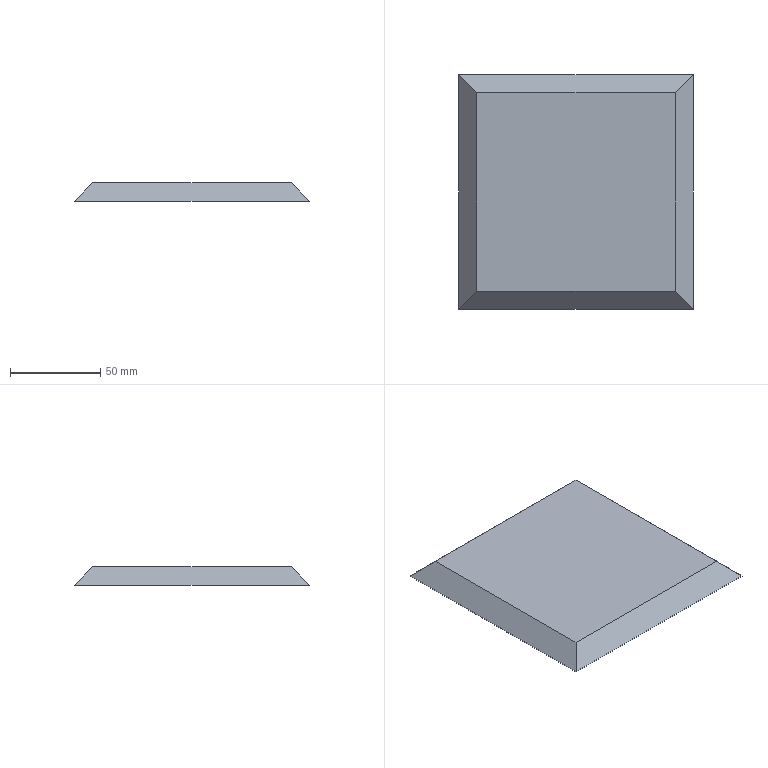Part | NX | features solid 2 | 1 solid | 6 faces | box 130 x 130 x 10 mm | volume 144333 mm3 | plane 6
STEP:
#1=CARTESIAN_POINT('',(-1255.,470.,-195.));
#2=VERTEX_POINT('',#1);
#3=CARTESIAN_POINT('',(-1145.,470.,-195.));
#4=VERTEX_POINT('',#3);
#5=CARTESIAN_POINT('',(-1095.,470.,-195.));
#6=DIRECTION('',(1.,0.,0.));
#7=VECTOR('',#6,1000.);
#8=LINE('',#5,#7);
#9=EDGE_CURVE('',#2,#4,#8,.T.);
#10=ORIENTED_EDGE('',*,*,#9,.T.);
#11=CARTESIAN_POINT('',(-1145.,580.,-195.));
#12=VERTEX_POINT('',#11);
#13=CARTESIAN_POINT('',(-1145.,420.,-195.));
#14=DIRECTION('',(0.,1.,0.));
#15=VECTOR('',#14,1000.);
#16=LINE('',#13,#15);
#17=EDGE_CURVE('',#4,#12,#16,.T.);
#18=ORIENTED_EDGE('',*,*,#17,.T.);
#19=CARTESIAN_POINT('',(-1255.,580.,-195.));
#20=VERTEX_POINT('',#19);
#21=CARTESIAN_POINT('',(-1095.,580.,-195.));
#22=DIRECTION('',(-1.,0.,0.));
#23=VECTOR('',#22,1000.);
#24=LINE('',#21,#23);
#25=EDGE_CURVE('',#12,#20,#24,.T.);
#26=ORIENTED_EDGE('',*,*,#25,.T.);
#27=CARTESIAN_POINT('',(-1255.,420.,-195.));
#28=DIRECTION('',(0.,-1.,0.));
#29=VECTOR('',#28,1000.);
#30=LINE('',#27,#29);
#31=EDGE_CURVE('',#20,#2,#30,.T.);
#32=ORIENTED_EDGE('',*,*,#31,.T.);
#33=EDGE_LOOP('',(#10,#18,#26,#32));
#34=FACE_BOUND('',#33,.T.);
#35=CARTESIAN_POINT('',(-1095.,420.,-195.));
#36=DIRECTION('',(0.,0.,-1.));
#37=DIRECTION('',(-1.,0.,0.));
#38=AXIS2_PLACEMENT_3D('',#35,#36,#37);
#39=PLANE('',#38);
#40=ADVANCED_FACE('',(#34),#39,.F.);
#41=CARTESIAN_POINT('',(-1135.,460.,-205.));
#42=VERTEX_POINT('',#41);
#43=CARTESIAN_POINT('',(-1135.,590.,-205.));
#44=VERTEX_POINT('',#43);
#45=CARTESIAN_POINT('',(-1135.,420.,-205.));
#46=DIRECTION('',(0.,1.,0.));
#47=VECTOR('',#46,1000.);
#48=LINE('',#45,#47);
#49=EDGE_CURVE('',#42,#44,#48,.T.);
#50=ORIENTED_EDGE('',*,*,#49,.F.);
#51=CARTESIAN_POINT('',(-1265.,460.,-205.));
#52=VERTEX_POINT('',#51);
#53=CARTESIAN_POINT('',(-1095.,460.,-205.));
#54=DIRECTION('',(1.,0.,0.));
#55=VECTOR('',#54,1000.);
#56=LINE('',#53,#55);
#57=EDGE_CURVE('',#52,#42,#56,.T.);
#58=ORIENTED_EDGE('',*,*,#57,.F.);
#59=CARTESIAN_POINT('',(-1265.,590.,-205.));
#60=VERTEX_POINT('',#59);
#61=CARTESIAN_POINT('',(-1265.,420.,-205.));
#62=DIRECTION('',(0.,-1.,0.));
#63=VECTOR('',#62,1000.);
#64=LINE('',#61,#63);
#65=EDGE_CURVE('',#60,#52,#64,.T.);
#66=ORIENTED_EDGE('',*,*,#65,.F.);
#67=CARTESIAN_POINT('',(-1095.,590.,-205.));
#68=DIRECTION('',(1.,0.,0.));
#69=VECTOR('',#68,1000.);
#70=LINE('',#67,#69);
#71=EDGE_CURVE('',#44,#60,#70,.F.);
#72=ORIENTED_EDGE('',*,*,#71,.F.);
#73=EDGE_LOOP('',(#50,#58,#66,#72));
#74=FACE_BOUND('',#73,.T.);
#75=CARTESIAN_POINT('',(-1095.,420.,-205.));
#76=DIRECTION('',(0.,0.,-1.));
#77=DIRECTION('',(-1.,0.,0.));
#78=AXIS2_PLACEMENT_3D('',#75,#76,#77);
#79=PLANE('',#78);
#80=ADVANCED_FACE('',(#74),#79,.T.);
#81=ORIENTED_EDGE('',*,*,#25,.F.);
#82=CARTESIAN_POINT('',(-1131.667,593.333,-208.333));
#83=DIRECTION('',(-0.5774,-0.5774,0.5774));
#84=VECTOR('',#83,1000.);
#85=LINE('',#82,#84);
#86=EDGE_CURVE('',#12,#44,#85,.F.);
#87=ORIENTED_EDGE('',*,*,#86,.T.);
#88=ORIENTED_EDGE('',*,*,#71,.T.);
#89=CARTESIAN_POINT('',(-1201.667,526.667,-141.667));
#90=DIRECTION('',(-0.5774,0.5774,-0.5774));
#91=VECTOR('',#90,1000.);
#92=LINE('',#89,#91);
#93=EDGE_CURVE('',#20,#60,#92,.T.);
#94=ORIENTED_EDGE('',*,*,#93,.F.);
#95=EDGE_LOOP('',(#81,#87,#88,#94));
#96=FACE_BOUND('',#95,.T.);
#97=CARTESIAN_POINT('',(-1095.,580.,-195.));
#98=DIRECTION('',(0.,0.7071,0.7071));
#99=DIRECTION('',(0.,0.7071,-0.7071));
#100=AXIS2_PLACEMENT_3D('',#97,#98,#99);
#101=PLANE('',#100);
#102=ADVANCED_FACE('',(#96),#101,.T.);
#103=ORIENTED_EDGE('',*,*,#93,.T.);
#104=ORIENTED_EDGE('',*,*,#65,.T.);
#105=CARTESIAN_POINT('',(-1268.333,456.667,-208.333));
#106=DIRECTION('',(0.5774,0.5774,0.5774));
#107=VECTOR('',#106,1000.);
#108=LINE('',#105,#107);
#109=EDGE_CURVE('',#2,#52,#108,.F.);
#110=ORIENTED_EDGE('',*,*,#109,.F.);
#111=ORIENTED_EDGE('',*,*,#31,.F.);
#112=EDGE_LOOP('',(#103,#104,#110,#111));
#113=FACE_BOUND('',#112,.T.);
#114=CARTESIAN_POINT('',(-1255.,420.,-195.));
#115=DIRECTION('',(0.7071,0.,-0.7071));
#116=DIRECTION('',(0.7071,0.,0.7071));
#117=AXIS2_PLACEMENT_3D('',#114,#115,#116);
#118=PLANE('',#117);
#119=ADVANCED_FACE('',(#113),#118,.F.);
#120=ORIENTED_EDGE('',*,*,#57,.T.);
#121=CARTESIAN_POINT('',(-1131.667,456.667,-208.333));
#122=DIRECTION('',(-0.5774,0.5774,0.5774));
#123=VECTOR('',#122,1000.);
#124=LINE('',#121,#123);
#125=EDGE_CURVE('',#42,#4,#124,.T.);
#126=ORIENTED_EDGE('',*,*,#125,.T.);
#127=ORIENTED_EDGE('',*,*,#9,.F.);
#128=ORIENTED_EDGE('',*,*,#109,.T.);
#129=EDGE_LOOP('',(#120,#126,#127,#128));
#130=FACE_BOUND('',#129,.T.);
#131=CARTESIAN_POINT('',(-1095.,470.,-195.));
#132=DIRECTION('',(0.,0.7071,-0.7071));
#133=DIRECTION('',(0.,-0.7071,-0.7071));
#134=AXIS2_PLACEMENT_3D('',#131,#132,#133);
#135=PLANE('',#134);
#136=ADVANCED_FACE('',(#130),#135,.F.);
#137=ORIENTED_EDGE('',*,*,#125,.F.);
#138=ORIENTED_EDGE('',*,*,#49,.T.);
#139=ORIENTED_EDGE('',*,*,#86,.F.);
#140=ORIENTED_EDGE('',*,*,#17,.F.);
#141=EDGE_LOOP('',(#137,#138,#139,#140));
#142=FACE_BOUND('',#141,.T.);
#143=CARTESIAN_POINT('',(-1145.,420.,-195.));
#144=DIRECTION('',(-0.7071,0.,-0.7071));
#145=DIRECTION('',(0.7071,0.,-0.7071));
#146=AXIS2_PLACEMENT_3D('',#143,#144,#145);
#147=PLANE('',#146);
#148=ADVANCED_FACE('',(#142),#147,.F.);
#149=CLOSED_SHELL('',(#40,#80,#102,#119,#136,#148));
#150=MANIFOLD_SOLID_BREP('',#149);
#151=(LENGTH_UNIT()NAMED_UNIT(*)SI_UNIT(.MILLI.,.METRE.));
#152=UNCERTAINTY_MEASURE_WITH_UNIT(LENGTH_MEASURE(0.00001),#151,'','');
#153=(NAMED_UNIT(*)PLANE_ANGLE_UNIT()SI_UNIT($,.RADIAN.));
#154=(NAMED_UNIT(*)SI_UNIT($,.STERADIAN.)SOLID_ANGLE_UNIT());
#155=(GEOMETRIC_REPRESENTATION_CONTEXT(3)GLOBAL_UNCERTAINTY_ASSIGNED_CONTEXT((#152))GLOBAL_UNIT_ASSIGNED_CONTEXT((#151,#153,#154))REPRESENTATION_CONTEXT('',''));
#156=ADVANCED_BREP_SHAPE_REPRESENTATION('',(#150),#155);